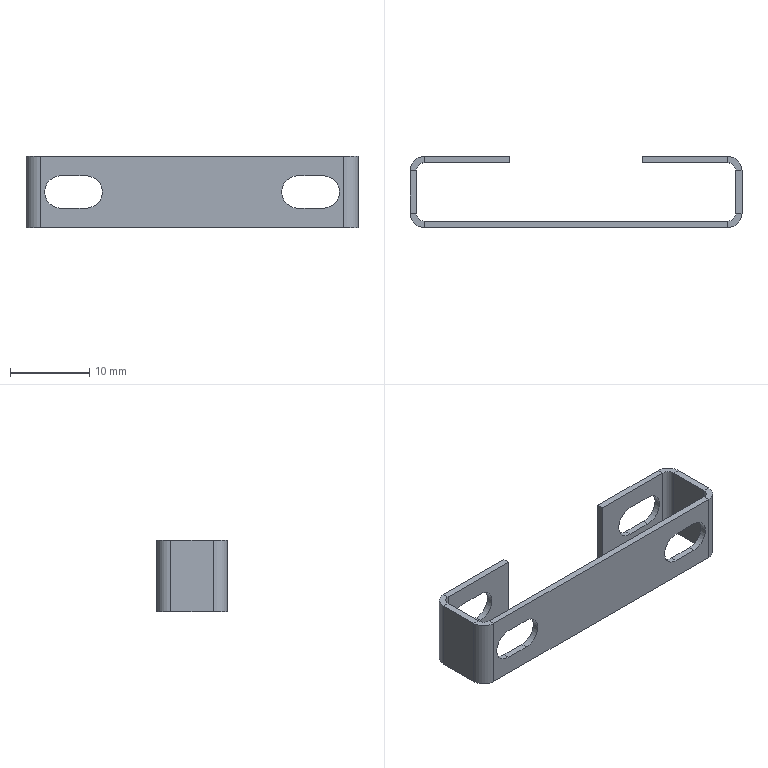Part | STEP file | KTC displacement sensor fixing sheet metal | 1 solid | 58 faces | box 42 x 9 x 9 mm | volume 488.862 mm3 | plane 38 | cylinder 20 | commonest cylinder face diameters 4.1 x12 2 x4 3.6 x4